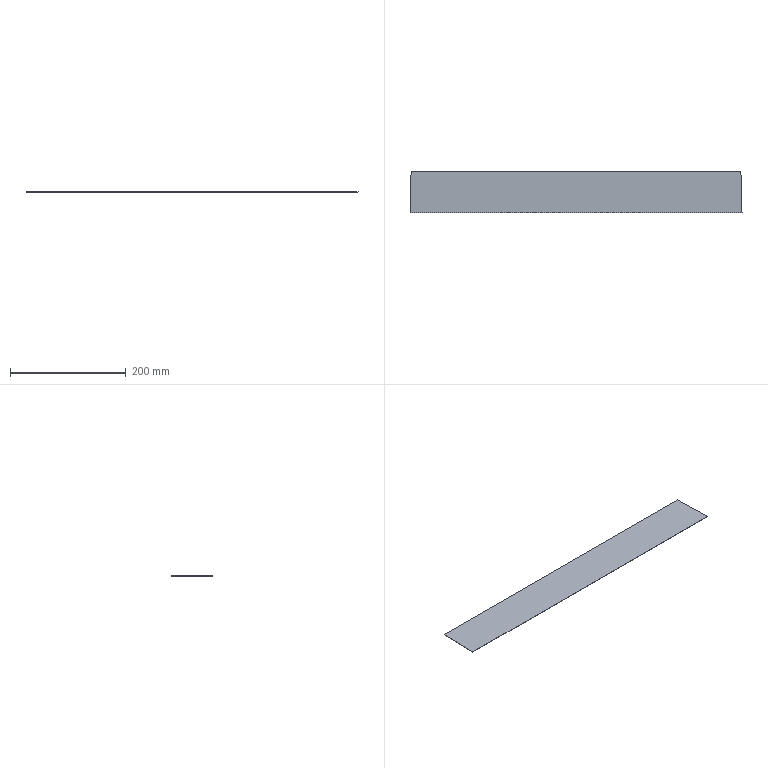Part | SolidWorks | features BaseBody 1 | 1 solid | 6 faces | box 572.8 x 71.5 x 0.5 mm | volume 20411 mm3 | plane 6
STEP:
#1=CARTESIAN_POINT('',(-286.4,-35.75,0.));
#2=VERTEX_POINT('',#1);
#3=CARTESIAN_POINT('',(-286.4,-35.75,0.5));
#4=VERTEX_POINT('',#3);
#5=CARTESIAN_POINT('',(-286.4,-35.75,0.25));
#6=DIRECTION('',(0.,0.,1.));
#7=VECTOR('',#6,1000.);
#8=LINE('',#5,#7);
#9=EDGE_CURVE('',#2,#4,#8,.T.);
#10=ORIENTED_EDGE('',*,*,#9,.T.);
#11=CARTESIAN_POINT('',(-284.528,35.75,0.5));
#12=VERTEX_POINT('',#11);
#13=CARTESIAN_POINT('',(-285.464,0.,0.5));
#14=DIRECTION('',(-0.02618,-0.9997,0.));
#15=VECTOR('',#14,1000.);
#16=LINE('',#13,#15);
#17=EDGE_CURVE('',#12,#4,#16,.T.);
#18=ORIENTED_EDGE('',*,*,#17,.F.);
#19=CARTESIAN_POINT('',(-284.528,35.75,0.));
#20=VERTEX_POINT('',#19);
#21=CARTESIAN_POINT('',(-284.528,35.75,0.25));
#22=DIRECTION('',(0.,0.,-1.));
#23=VECTOR('',#22,1000.);
#24=LINE('',#21,#23);
#25=EDGE_CURVE('',#12,#20,#24,.T.);
#26=ORIENTED_EDGE('',*,*,#25,.T.);
#27=CARTESIAN_POINT('',(-285.464,0.,0.));
#28=DIRECTION('',(0.02618,0.9997,0.));
#29=VECTOR('',#28,1000.);
#30=LINE('',#27,#29);
#31=EDGE_CURVE('',#2,#20,#30,.T.);
#32=ORIENTED_EDGE('',*,*,#31,.F.);
#33=EDGE_LOOP('',(#10,#18,#26,#32));
#34=FACE_OUTER_BOUND('',#33,.T.);
#35=CARTESIAN_POINT('',(-286.4,-35.75,0.));
#36=DIRECTION('',(0.9997,-0.02618,0.));
#37=DIRECTION('',(0.02618,0.9997,0.));
#38=AXIS2_PLACEMENT_3D('',#35,#36,#37);
#39=PLANE('',#38);
#40=ADVANCED_FACE('',(#34),#39,.F.);
#41=CARTESIAN_POINT('',(284.528,35.75,0.));
#42=VERTEX_POINT('',#41);
#43=CARTESIAN_POINT('',(286.4,-35.75,0.));
#44=VERTEX_POINT('',#43);
#45=CARTESIAN_POINT('',(284.528,35.75,0.));
#46=DIRECTION('',(0.02618,-0.9997,0.));
#47=VECTOR('',#46,1000.);
#48=LINE('',#45,#47);
#49=EDGE_CURVE('',#42,#44,#48,.T.);
#50=ORIENTED_EDGE('',*,*,#49,.T.);
#51=CARTESIAN_POINT('',(0.,-35.75,0.));
#52=DIRECTION('',(-1.,0.,0.));
#53=VECTOR('',#52,1000.);
#54=LINE('',#51,#53);
#55=EDGE_CURVE('',#44,#2,#54,.T.);
#56=ORIENTED_EDGE('',*,*,#55,.T.);
#57=ORIENTED_EDGE('',*,*,#31,.T.);
#58=CARTESIAN_POINT('',(0.,35.75,0.));
#59=DIRECTION('',(1.,0.,0.));
#60=VECTOR('',#59,1000.);
#61=LINE('',#58,#60);
#62=EDGE_CURVE('',#20,#42,#61,.T.);
#63=ORIENTED_EDGE('',*,*,#62,.T.);
#64=EDGE_LOOP('',(#50,#56,#57,#63));
#65=FACE_OUTER_BOUND('',#64,.T.);
#66=CARTESIAN_POINT('',(289.837,-35.75,0.));
#67=DIRECTION('',(0.,0.,-1.));
#68=DIRECTION('',(-1.,0.,0.));
#69=AXIS2_PLACEMENT_3D('',#66,#67,#68);
#70=PLANE('',#69);
#71=ADVANCED_FACE('',(#65),#70,.T.);
#72=CARTESIAN_POINT('',(286.4,-35.75,0.5));
#73=VERTEX_POINT('',#72);
#74=CARTESIAN_POINT('',(0.,-35.75,0.5));
#75=DIRECTION('',(-1.,0.,0.));
#76=VECTOR('',#75,1000.);
#77=LINE('',#74,#76);
#78=EDGE_CURVE('',#73,#4,#77,.T.);
#79=ORIENTED_EDGE('',*,*,#78,.F.);
#80=CARTESIAN_POINT('',(284.528,35.75,0.5));
#81=VERTEX_POINT('',#80);
#82=CARTESIAN_POINT('',(284.528,35.75,0.5));
#83=DIRECTION('',(0.02618,-0.9997,0.));
#84=VECTOR('',#83,1000.);
#85=LINE('',#82,#84);
#86=EDGE_CURVE('',#81,#73,#85,.T.);
#87=ORIENTED_EDGE('',*,*,#86,.F.);
#88=CARTESIAN_POINT('',(0.,35.75,0.5));
#89=DIRECTION('',(1.,0.,0.));
#90=VECTOR('',#89,1000.);
#91=LINE('',#88,#90);
#92=EDGE_CURVE('',#12,#81,#91,.T.);
#93=ORIENTED_EDGE('',*,*,#92,.F.);
#94=ORIENTED_EDGE('',*,*,#17,.T.);
#95=EDGE_LOOP('',(#79,#87,#93,#94));
#96=FACE_OUTER_BOUND('',#95,.T.);
#97=CARTESIAN_POINT('',(289.837,-35.75,0.5));
#98=DIRECTION('',(0.,0.,-1.));
#99=DIRECTION('',(-1.,0.,0.));
#100=AXIS2_PLACEMENT_3D('',#97,#98,#99);
#101=PLANE('',#100);
#102=ADVANCED_FACE('',(#96),#101,.F.);
#103=CARTESIAN_POINT('',(286.4,-35.75,0.25));
#104=DIRECTION('',(0.,0.,-1.));
#105=VECTOR('',#104,1000.);
#106=LINE('',#103,#105);
#107=EDGE_CURVE('',#73,#44,#106,.T.);
#108=ORIENTED_EDGE('',*,*,#107,.F.);
#109=ORIENTED_EDGE('',*,*,#78,.T.);
#110=ORIENTED_EDGE('',*,*,#9,.F.);
#111=ORIENTED_EDGE('',*,*,#55,.F.);
#112=EDGE_LOOP('',(#108,#109,#110,#111));
#113=FACE_OUTER_BOUND('',#112,.T.);
#114=CARTESIAN_POINT('',(-286.4,-35.75,0.));
#115=DIRECTION('',(0.,1.,0.));
#116=DIRECTION('',(0.,0.,1.));
#117=AXIS2_PLACEMENT_3D('',#114,#115,#116);
#118=PLANE('',#117);
#119=ADVANCED_FACE('',(#113),#118,.F.);
#120=CARTESIAN_POINT('',(284.528,35.75,0.25));
#121=DIRECTION('',(0.,0.,-1.));
#122=VECTOR('',#121,1000.);
#123=LINE('',#120,#122);
#124=EDGE_CURVE('',#81,#42,#123,.T.);
#125=ORIENTED_EDGE('',*,*,#124,.F.);
#126=ORIENTED_EDGE('',*,*,#86,.T.);
#127=ORIENTED_EDGE('',*,*,#107,.T.);
#128=ORIENTED_EDGE('',*,*,#49,.F.);
#129=EDGE_LOOP('',(#125,#126,#127,#128));
#130=FACE_OUTER_BOUND('',#129,.T.);
#131=CARTESIAN_POINT('',(284.528,35.75,0.));
#132=DIRECTION('',(-0.9997,-0.02618,0.));
#133=DIRECTION('',(0.02618,-0.9997,0.));
#134=AXIS2_PLACEMENT_3D('',#131,#132,#133);
#135=PLANE('',#134);
#136=ADVANCED_FACE('',(#130),#135,.F.);
#137=ORIENTED_EDGE('',*,*,#25,.F.);
#138=ORIENTED_EDGE('',*,*,#92,.T.);
#139=ORIENTED_EDGE('',*,*,#124,.T.);
#140=ORIENTED_EDGE('',*,*,#62,.F.);
#141=EDGE_LOOP('',(#137,#138,#139,#140));
#142=FACE_OUTER_BOUND('',#141,.T.);
#143=CARTESIAN_POINT('',(-284.528,35.75,0.5));
#144=DIRECTION('',(0.,-1.,0.));
#145=DIRECTION('',(0.,0.,-1.));
#146=AXIS2_PLACEMENT_3D('',#143,#144,#145);
#147=PLANE('',#146);
#148=ADVANCED_FACE('',(#142),#147,.F.);
#149=CLOSED_SHELL('',(#40,#71,#102,#119,#136,#148));
#150=MANIFOLD_SOLID_BREP('',#149);
#151=CARTESIAN_POINT('',(0.,0.,0.));
#152=DIRECTION('',(0.,0.,1.));
#153=DIRECTION('',(1.,0.,0.));
#154=AXIS2_PLACEMENT_3D('',#151,#152,#153);
#155=(LENGTH_UNIT()NAMED_UNIT(*)SI_UNIT(.MILLI.,.METRE.));
#156=UNCERTAINTY_MEASURE_WITH_UNIT(LENGTH_MEASURE(0.00001),#155,'','');
#157=(NAMED_UNIT(*)PLANE_ANGLE_UNIT()SI_UNIT($,.RADIAN.));
#158=(NAMED_UNIT(*)SI_UNIT($,.STERADIAN.)SOLID_ANGLE_UNIT());
#159=(GEOMETRIC_REPRESENTATION_CONTEXT(3)GLOBAL_UNCERTAINTY_ASSIGNED_CONTEXT((#156))GLOBAL_UNIT_ASSIGNED_CONTEXT((#155,#157,#158))REPRESENTATION_CONTEXT('',''));
#160=ADVANCED_BREP_SHAPE_REPRESENTATION('',(#150,#154),#159);